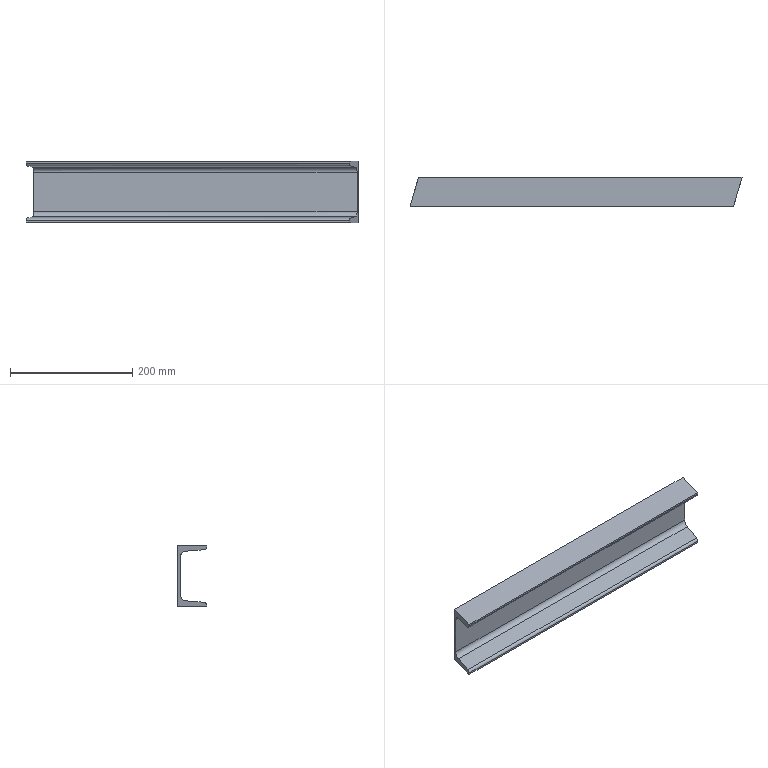Part | STEP file | 12-Channel 100x48_default<machining> | 1 solid | 14 faces | box 544 x 48 x 100 mm | volume 666800 mm3 | plane 10 | cylinder 4 | commonest cylinder face diameters 8.5 x2 17 x2
STEP:
#1=CARTESIAN_POINT('',(0.,0.,0.));
#2=DIRECTION('',(0.,0.,1.));
#3=DIRECTION('',(1.,0.,0.));
#4=AXIS2_PLACEMENT_3D('',#1,#2,#3);
#5=CARTESIAN_POINT('',(544.,0.,-100.));
#6=VERTEX_POINT('',#5);
#7=CARTESIAN_POINT('',(14.,0.,-100.));
#8=VERTEX_POINT('',#7);
#9=CARTESIAN_POINT('',(544.,0.,-100.));
#10=DIRECTION('',(-1.,0.,0.));
#11=VECTOR('',#10,1.);
#12=LINE('',#9,#11);
#13=CARTESIAN_POINT('',(544.,0.,-100.));
#14=DIRECTION('',(0.,0.,1.));
#15=DIRECTION('',(1.,0.,0.));
#16=AXIS2_PLACEMENT_3D('',#13,#14,#15);
#17=PLANE('',#16);
#18=CARTESIAN_POINT('',(0.,0.));
#19=DIRECTION('',(-1.,0.));
#20=VECTOR('',#19,1.);
#21=LINE('',#18,#20);
#22=(GEOMETRIC_REPRESENTATION_CONTEXT(2)PARAMETRIC_REPRESENTATION_CONTEXT()REPRESENTATION_CONTEXT('',''));
#23=DEFINITIONAL_REPRESENTATION('',(#21),#22);
#24=PCURVE('',#17,#23);
#25=CARTESIAN_POINT('',(544.,0.,0.));
#26=DIRECTION('',(0.,-1.,0.));
#27=DIRECTION('',(0.,0.,-1.));
#28=AXIS2_PLACEMENT_3D('',#25,#26,#27);
#29=PLANE('',#28);
#30=CARTESIAN_POINT('',(100.,0.));
#31=DIRECTION('',(0.,-1.));
#32=VECTOR('',#31,1.);
#33=LINE('',#30,#32);
#34=(GEOMETRIC_REPRESENTATION_CONTEXT(2)PARAMETRIC_REPRESENTATION_CONTEXT()REPRESENTATION_CONTEXT('',''));
#35=DEFINITIONAL_REPRESENTATION('',(#33),#34);
#36=PCURVE('',#29,#35);
#37=SURFACE_CURVE('',#12,(#24,#36),.PCURVE_S1.);
#38=EDGE_CURVE('',#6,#8,#37,.T.);
#39=ORIENTED_EDGE('',*,*,#38,.F.);
#40=CARTESIAN_POINT('',(530.,-48.,-100.));
#41=VERTEX_POINT('',#40);
#42=CARTESIAN_POINT('',(544.,0.,-100.));
#43=DIRECTION('',(0.28,0.96,0.));
#44=VECTOR('',#43,1.);
#45=LINE('',#42,#44);
#46=CARTESIAN_POINT('',(0.,0.));
#47=DIRECTION('',(0.28,0.96));
#48=VECTOR('',#47,1.);
#49=LINE('',#46,#48);
#50=(GEOMETRIC_REPRESENTATION_CONTEXT(2)PARAMETRIC_REPRESENTATION_CONTEXT()REPRESENTATION_CONTEXT('',''));
#51=DEFINITIONAL_REPRESENTATION('',(#49),#50);
#52=PCURVE('',#17,#51);
#53=CARTESIAN_POINT('',(544.,0.,0.));
#54=DIRECTION('',(-0.96,0.28,0.));
#55=DIRECTION('',(-0.28,-0.96,0.));
#56=AXIS2_PLACEMENT_3D('',#53,#54,#55);
#57=PLANE('',#56);
#58=CARTESIAN_POINT('',(0.,-100.));
#59=DIRECTION('',(-1.,0.));
#60=VECTOR('',#59,1.);
#61=LINE('',#58,#60);
#62=(GEOMETRIC_REPRESENTATION_CONTEXT(2)PARAMETRIC_REPRESENTATION_CONTEXT()REPRESENTATION_CONTEXT('',''));
#63=DEFINITIONAL_REPRESENTATION('',(#61),#62);
#64=PCURVE('',#57,#63);
#65=SURFACE_CURVE('',#45,(#52,#64),.PCURVE_S1.);
#66=EDGE_CURVE('',#41,#6,#65,.T.);
#67=ORIENTED_EDGE('',*,*,#66,.F.);
#68=CARTESIAN_POINT('',(0.,-48.,-100.));
#69=VERTEX_POINT('',#68);
#70=CARTESIAN_POINT('',(544.,-48.,-100.));
#71=DIRECTION('',(-1.,0.,0.));
#72=VECTOR('',#71,1.);
#73=LINE('',#70,#72);
#74=CARTESIAN_POINT('',(0.,-48.));
#75=DIRECTION('',(-1.,0.));
#76=VECTOR('',#75,1.);
#77=LINE('',#74,#76);
#78=(GEOMETRIC_REPRESENTATION_CONTEXT(2)PARAMETRIC_REPRESENTATION_CONTEXT()REPRESENTATION_CONTEXT('',''));
#79=DEFINITIONAL_REPRESENTATION('',(#77),#78);
#80=PCURVE('',#17,#79);
#81=CARTESIAN_POINT('',(544.,-48.,-97.266));
#82=DIRECTION('',(0.,1.,0.));
#83=DIRECTION('',(0.,0.,1.));
#84=AXIS2_PLACEMENT_3D('',#81,#82,#83);
#85=PLANE('',#84);
#86=CARTESIAN_POINT('',(-2.734,0.));
#87=DIRECTION('',(0.,-1.));
#88=VECTOR('',#87,1.);
#89=LINE('',#86,#88);
#90=(GEOMETRIC_REPRESENTATION_CONTEXT(2)PARAMETRIC_REPRESENTATION_CONTEXT()REPRESENTATION_CONTEXT('',''));
#91=DEFINITIONAL_REPRESENTATION('',(#89),#90);
#92=PCURVE('',#85,#91);
#93=SURFACE_CURVE('',#73,(#80,#92),.PCURVE_S1.);
#94=EDGE_CURVE('',#41,#69,#93,.T.);
#95=ORIENTED_EDGE('',*,*,#94,.T.);
#96=CARTESIAN_POINT('',(0.,-48.,-100.));
#97=DIRECTION('',(-0.28,-0.96,0.));
#98=VECTOR('',#97,1.);
#99=LINE('',#96,#98);
#100=CARTESIAN_POINT('',(-544.,-48.));
#101=DIRECTION('',(-0.28,-0.96));
#102=VECTOR('',#101,1.);
#103=LINE('',#100,#102);
#104=(GEOMETRIC_REPRESENTATION_CONTEXT(2)PARAMETRIC_REPRESENTATION_CONTEXT()REPRESENTATION_CONTEXT('',''));
#105=DEFINITIONAL_REPRESENTATION('',(#103),#104);
#106=PCURVE('',#17,#105);
#107=CARTESIAN_POINT('',(0.,-48.,0.));
#108=DIRECTION('',(0.96,-0.28,0.));
#109=DIRECTION('',(0.28,0.96,0.));
#110=AXIS2_PLACEMENT_3D('',#107,#108,#109);
#111=PLANE('',#110);
#112=CARTESIAN_POINT('',(0.,-100.));
#113=DIRECTION('',(-1.,0.));
#114=VECTOR('',#113,1.);
#115=LINE('',#112,#114);
#116=(GEOMETRIC_REPRESENTATION_CONTEXT(2)PARAMETRIC_REPRESENTATION_CONTEXT()REPRESENTATION_CONTEXT('',''));
#117=DEFINITIONAL_REPRESENTATION('',(#115),#116);
#118=PCURVE('',#111,#117);
#119=SURFACE_CURVE('',#99,(#106,#118),.PCURVE_S1.);
#120=EDGE_CURVE('',#8,#69,#119,.T.);
#121=ORIENTED_EDGE('',*,*,#120,.F.);
#122=EDGE_LOOP('',(#39,#67,#95,#121));
#123=FACE_BOUND('',#122,.T.);
#124=ADVANCED_FACE('',(#123),#17,.F.);
#125=ORIENTED_EDGE('',*,*,#38,.T.);
#126=CARTESIAN_POINT('',(14.,0.,0.));
#127=VERTEX_POINT('',#126);
#128=CARTESIAN_POINT('',(14.,0.,0.));
#129=DIRECTION('',(0.,0.,-1.));
#130=VECTOR('',#129,1.);
#131=LINE('',#128,#130);
#132=CARTESIAN_POINT('',(0.,-530.));
#133=DIRECTION('',(1.,0.));
#134=VECTOR('',#133,1.);
#135=LINE('',#132,#134);
#136=(GEOMETRIC_REPRESENTATION_CONTEXT(2)PARAMETRIC_REPRESENTATION_CONTEXT()REPRESENTATION_CONTEXT('',''));
#137=DEFINITIONAL_REPRESENTATION('',(#135),#136);
#138=PCURVE('',#29,#137);
#139=CARTESIAN_POINT('',(50.,0.));
#140=DIRECTION('',(0.,-1.));
#141=VECTOR('',#140,1.);
#142=LINE('',#139,#141);
#143=(GEOMETRIC_REPRESENTATION_CONTEXT(2)PARAMETRIC_REPRESENTATION_CONTEXT()REPRESENTATION_CONTEXT('',''));
#144=DEFINITIONAL_REPRESENTATION('',(#142),#143);
#145=PCURVE('',#111,#144);
#146=SURFACE_CURVE('',#131,(#138,#145),.PCURVE_S1.);
#147=EDGE_CURVE('',#127,#8,#146,.T.);
#148=ORIENTED_EDGE('',*,*,#147,.F.);
#149=CARTESIAN_POINT('',(544.,0.,0.));
#150=VERTEX_POINT('',#149);
#151=CARTESIAN_POINT('',(544.,0.,0.));
#152=DIRECTION('',(-1.,0.,0.));
#153=VECTOR('',#152,1.);
#154=LINE('',#151,#153);
#155=CARTESIAN_POINT('',(0.,0.));
#156=DIRECTION('',(0.,-1.));
#157=VECTOR('',#156,1.);
#158=LINE('',#155,#157);
#159=(GEOMETRIC_REPRESENTATION_CONTEXT(2)PARAMETRIC_REPRESENTATION_CONTEXT()REPRESENTATION_CONTEXT('',''));
#160=DEFINITIONAL_REPRESENTATION('',(#158),#159);
#161=PCURVE('',#29,#160);
#162=CARTESIAN_POINT('',(544.,0.,0.));
#163=DIRECTION('',(0.,0.,-1.));
#164=DIRECTION('',(0.,1.,0.));
#165=AXIS2_PLACEMENT_3D('',#162,#163,#164);
#166=PLANE('',#165);
#167=CARTESIAN_POINT('',(0.,0.));
#168=DIRECTION('',(0.,-1.));
#169=VECTOR('',#168,1.);
#170=LINE('',#167,#169);
#171=(GEOMETRIC_REPRESENTATION_CONTEXT(2)PARAMETRIC_REPRESENTATION_CONTEXT()REPRESENTATION_CONTEXT('',''));
#172=DEFINITIONAL_REPRESENTATION('',(#170),#171);
#173=PCURVE('',#166,#172);
#174=SURFACE_CURVE('',#154,(#161,#173),.PCURVE_S1.);
#175=EDGE_CURVE('',#150,#127,#174,.T.);
#176=ORIENTED_EDGE('',*,*,#175,.F.);
#177=CARTESIAN_POINT('',(544.,0.,0.));
#178=DIRECTION('',(0.,0.,1.));
#179=VECTOR('',#178,1.);
#180=LINE('',#177,#179);
#181=CARTESIAN_POINT('',(0.,0.));
#182=DIRECTION('',(-1.,0.));
#183=VECTOR('',#182,1.);
#184=LINE('',#181,#183);
#185=(GEOMETRIC_REPRESENTATION_CONTEXT(2)PARAMETRIC_REPRESENTATION_CONTEXT()REPRESENTATION_CONTEXT('',''));
#186=DEFINITIONAL_REPRESENTATION('',(#184),#185);
#187=PCURVE('',#29,#186);
#188=CARTESIAN_POINT('',(0.,0.));
#189=DIRECTION('',(0.,1.));
#190=VECTOR('',#189,1.);
#191=LINE('',#188,#190);
#192=(GEOMETRIC_REPRESENTATION_CONTEXT(2)PARAMETRIC_REPRESENTATION_CONTEXT()REPRESENTATION_CONTEXT('',''));
#193=DEFINITIONAL_REPRESENTATION('',(#191),#192);
#194=PCURVE('',#57,#193);
#195=SURFACE_CURVE('',#180,(#187,#194),.PCURVE_S1.);
#196=EDGE_CURVE('',#6,#150,#195,.T.);
#197=ORIENTED_EDGE('',*,*,#196,.F.);
#198=EDGE_LOOP('',(#125,#148,#176,#197));
#199=FACE_BOUND('',#198,.T.);
#200=ADVANCED_FACE('',(#199),#29,.F.);
#201=CARTESIAN_POINT('',(530.,-48.,0.));
#202=VERTEX_POINT('',#201);
#203=CARTESIAN_POINT('',(0.,-48.,0.));
#204=VERTEX_POINT('',#203);
#205=CARTESIAN_POINT('',(544.,-48.,0.));
#206=DIRECTION('',(-1.,0.,0.));
#207=VECTOR('',#206,1.);
#208=LINE('',#205,#207);
#209=CARTESIAN_POINT('',(-48.,0.));
#210=DIRECTION('',(0.,-1.));
#211=VECTOR('',#210,1.);
#212=LINE('',#209,#211);
#213=(GEOMETRIC_REPRESENTATION_CONTEXT(2)PARAMETRIC_REPRESENTATION_CONTEXT()REPRESENTATION_CONTEXT('',''));
#214=DEFINITIONAL_REPRESENTATION('',(#212),#213);
#215=PCURVE('',#166,#214);
#216=CARTESIAN_POINT('',(544.,-48.,-2.734));
#217=DIRECTION('',(0.,1.,0.));
#218=DIRECTION('',(0.,0.,1.));
#219=AXIS2_PLACEMENT_3D('',#216,#217,#218);
#220=PLANE('',#219);
#221=CARTESIAN_POINT('',(2.734,0.));
#222=DIRECTION('',(0.,-1.));
#223=VECTOR('',#222,1.);
#224=LINE('',#221,#223);
#225=(GEOMETRIC_REPRESENTATION_CONTEXT(2)PARAMETRIC_REPRESENTATION_CONTEXT()REPRESENTATION_CONTEXT('',''));
#226=DEFINITIONAL_REPRESENTATION('',(#224),#225);
#227=PCURVE('',#220,#226);
#228=SURFACE_CURVE('',#208,(#215,#227),.PCURVE_S1.);
#229=EDGE_CURVE('',#202,#204,#228,.T.);
#230=ORIENTED_EDGE('',*,*,#229,.F.);
#231=CARTESIAN_POINT('',(544.,0.,0.));
#232=DIRECTION('',(0.28,0.96,0.));
#233=VECTOR('',#232,1.);
#234=LINE('',#231,#233);
#235=CARTESIAN_POINT('',(0.,0.));
#236=DIRECTION('',(0.96,0.28));
#237=VECTOR('',#236,1.);
#238=LINE('',#235,#237);
#239=(GEOMETRIC_REPRESENTATION_CONTEXT(2)PARAMETRIC_REPRESENTATION_CONTEXT()REPRESENTATION_CONTEXT('',''));
#240=DEFINITIONAL_REPRESENTATION('',(#238),#239);
#241=PCURVE('',#166,#240);
#242=CARTESIAN_POINT('',(0.,0.));
#243=DIRECTION('',(-1.,0.));
#244=VECTOR('',#243,1.);
#245=LINE('',#242,#244);
#246=(GEOMETRIC_REPRESENTATION_CONTEXT(2)PARAMETRIC_REPRESENTATION_CONTEXT()REPRESENTATION_CONTEXT('',''));
#247=DEFINITIONAL_REPRESENTATION('',(#245),#246);
#248=PCURVE('',#57,#247);
#249=SURFACE_CURVE('',#234,(#241,#248),.PCURVE_S1.);
#250=EDGE_CURVE('',#202,#150,#249,.T.);
#251=ORIENTED_EDGE('',*,*,#250,.T.);
#252=ORIENTED_EDGE('',*,*,#175,.T.);
#253=CARTESIAN_POINT('',(0.,-48.,0.));
#254=DIRECTION('',(-0.28,-0.96,0.));
#255=VECTOR('',#254,1.);
#256=LINE('',#253,#255);
#257=CARTESIAN_POINT('',(-48.,-544.));
#258=DIRECTION('',(-0.96,-0.28));
#259=VECTOR('',#258,1.);
#260=LINE('',#257,#259);
#261=(GEOMETRIC_REPRESENTATION_CONTEXT(2)PARAMETRIC_REPRESENTATION_CONTEXT()REPRESENTATION_CONTEXT('',''));
#262=DEFINITIONAL_REPRESENTATION('',(#260),#261);
#263=PCURVE('',#166,#262);
#264=CARTESIAN_POINT('',(0.,0.));
#265=DIRECTION('',(-1.,0.));
#266=VECTOR('',#265,1.);
#267=LINE('',#264,#266);
#268=(GEOMETRIC_REPRESENTATION_CONTEXT(2)PARAMETRIC_REPRESENTATION_CONTEXT()REPRESENTATION_CONTEXT('',''));
#269=DEFINITIONAL_REPRESENTATION('',(#267),#268);
#270=PCURVE('',#111,#269);
#271=SURFACE_CURVE('',#256,(#263,#270),.PCURVE_S1.);
#272=EDGE_CURVE('',#127,#204,#271,.T.);
#273=ORIENTED_EDGE('',*,*,#272,.T.);
#274=EDGE_LOOP('',(#230,#251,#252,#273));
#275=FACE_BOUND('',#274,.T.);
#276=ADVANCED_FACE('',(#275),#166,.F.);
#277=CARTESIAN_POINT('',(530.,-48.,-2.734));
#278=VERTEX_POINT('',#277);
#279=CARTESIAN_POINT('',(0.,-48.,-2.734));
#280=VERTEX_POINT('',#279);
#281=CARTESIAN_POINT('',(544.,-48.,-2.734));
#282=DIRECTION('',(-1.,0.,0.));
#283=VECTOR('',#282,1.);
#284=LINE('',#281,#283);
#285=CARTESIAN_POINT('',(0.,0.));
#286=DIRECTION('',(0.,-1.));
#287=VECTOR('',#286,1.);
#288=LINE('',#285,#287);
#289=(GEOMETRIC_REPRESENTATION_CONTEXT(2)PARAMETRIC_REPRESENTATION_CONTEXT()REPRESENTATION_CONTEXT('',''));
#290=DEFINITIONAL_REPRESENTATION('',(#288),#289);
#291=PCURVE('',#220,#290);
#292=CARTESIAN_POINT('',(544.,-43.75,-2.734));
#293=DIRECTION('',(-1.,0.,0.));
#294=DIRECTION('',(0.,0.,1.));
#295=AXIS2_PLACEMENT_3D('',#292,#293,#294);
#296=CYLINDRICAL_SURFACE('',#295,4.25);
#297=CARTESIAN_POINT('',(4.712,0.));
#298=DIRECTION('',(0.,1.));
#299=VECTOR('',#298,1.);
#300=LINE('',#297,#299);
#301=(GEOMETRIC_REPRESENTATION_CONTEXT(2)PARAMETRIC_REPRESENTATION_CONTEXT()REPRESENTATION_CONTEXT('',''));
#302=DEFINITIONAL_REPRESENTATION('',(#300),#301);
#303=PCURVE('',#296,#302);
#304=SURFACE_CURVE('',#284,(#291,#303),.PCURVE_S1.);
#305=EDGE_CURVE('',#278,#280,#304,.T.);
#306=ORIENTED_EDGE('',*,*,#305,.F.);
#307=CARTESIAN_POINT('',(530.,-48.,0.));
#308=DIRECTION('',(0.,0.,-1.));
#309=VECTOR('',#308,1.);
#310=LINE('',#307,#309);
#311=CARTESIAN_POINT('',(2.734,-14.));
#312=DIRECTION('',(-1.,0.));
#313=VECTOR('',#312,1.);
#314=LINE('',#311,#313);
#315=(GEOMETRIC_REPRESENTATION_CONTEXT(2)PARAMETRIC_REPRESENTATION_CONTEXT()REPRESENTATION_CONTEXT('',''));
#316=DEFINITIONAL_REPRESENTATION('',(#314),#315);
#317=PCURVE('',#220,#316);
#318=CARTESIAN_POINT('',(50.,0.));
#319=DIRECTION('',(0.,-1.));
#320=VECTOR('',#319,1.);
#321=LINE('',#318,#320);
#322=(GEOMETRIC_REPRESENTATION_CONTEXT(2)PARAMETRIC_REPRESENTATION_CONTEXT()REPRESENTATION_CONTEXT('',''));
#323=DEFINITIONAL_REPRESENTATION('',(#321),#322);
#324=PCURVE('',#57,#323);
#325=SURFACE_CURVE('',#310,(#317,#324),.PCURVE_S1.);
#326=EDGE_CURVE('',#202,#278,#325,.T.);
#327=ORIENTED_EDGE('',*,*,#326,.F.);
#328=ORIENTED_EDGE('',*,*,#229,.T.);
#329=CARTESIAN_POINT('',(0.,-48.,-2.734));
#330=DIRECTION('',(0.,0.,-1.));
#331=VECTOR('',#330,1.);
#332=LINE('',#329,#331);
#333=CARTESIAN_POINT('',(0.,-544.));
#334=DIRECTION('',(-1.,0.));
#335=VECTOR('',#334,1.);
#336=LINE('',#333,#335);
#337=(GEOMETRIC_REPRESENTATION_CONTEXT(2)PARAMETRIC_REPRESENTATION_CONTEXT()REPRESENTATION_CONTEXT('',''));
#338=DEFINITIONAL_REPRESENTATION('',(#336),#337);
#339=PCURVE('',#220,#338);
#340=CARTESIAN_POINT('',(0.,-2.734));
#341=DIRECTION('',(0.,-1.));
#342=VECTOR('',#341,1.);
#343=LINE('',#340,#342);
#344=(GEOMETRIC_REPRESENTATION_CONTEXT(2)PARAMETRIC_REPRESENTATION_CONTEXT()REPRESENTATION_CONTEXT('',''));
#345=DEFINITIONAL_REPRESENTATION('',(#343),#344);
#346=PCURVE('',#111,#345);
#347=SURFACE_CURVE('',#332,(#339,#346),.PCURVE_S1.);
#348=EDGE_CURVE('',#204,#280,#347,.T.);
#349=ORIENTED_EDGE('',*,*,#348,.T.);
#350=EDGE_LOOP('',(#306,#327,#328,#349));
#351=FACE_BOUND('',#350,.T.);
#352=ADVANCED_FACE('',(#351),#220,.F.);
#353=CARTESIAN_POINT('',(531.146,-44.073,-6.972));
#354=VERTEX_POINT('',#353);
#355=CARTESIAN_POINT('',(1.146,-44.073,-6.972));
#356=VERTEX_POINT('',#355);
#357=CARTESIAN_POINT('',(544.,-44.073,-6.972));
#358=DIRECTION('',(-1.,0.,0.));
#359=VECTOR('',#358,1.);
#360=LINE('',#357,#359);
#361=CARTESIAN_POINT('',(3.218,0.));
#362=DIRECTION('',(0.,1.));
#363=VECTOR('',#362,1.);
#364=LINE('',#361,#363);
#365=(GEOMETRIC_REPRESENTATION_CONTEXT(2)PARAMETRIC_REPRESENTATION_CONTEXT()REPRESENTATION_CONTEXT('',''));
#366=DEFINITIONAL_REPRESENTATION('',(#364),#365);
#367=PCURVE('',#296,#366);
#368=CARTESIAN_POINT('',(544.,-13.155,-9.325));
#369=DIRECTION('',(0.,0.07589,0.9971));
#370=DIRECTION('',(0.,-0.9971,0.07589));
#371=AXIS2_PLACEMENT_3D('',#368,#369,#370);
#372=PLANE('',#371);
#373=CARTESIAN_POINT('',(31.007,0.));
#374=DIRECTION('',(0.,-1.));
#375=VECTOR('',#374,1.);
#376=LINE('',#373,#375);
#377=(GEOMETRIC_REPRESENTATION_CONTEXT(2)PARAMETRIC_REPRESENTATION_CONTEXT()REPRESENTATION_CONTEXT('',''));
#378=DEFINITIONAL_REPRESENTATION('',(#376),#377);
#379=PCURVE('',#372,#378);
#380=SURFACE_CURVE('',#360,(#367,#379),.PCURVE_S1.);
#381=EDGE_CURVE('',#354,#356,#380,.T.);
#382=ORIENTED_EDGE('',*,*,#381,.F.);
#383=CARTESIAN_POINT('',(531.146,-44.073,-6.972));
#384=CARTESIAN_POINT('',(530.464,-46.408,-6.794));
#385=CARTESIAN_POINT('',(530.,-48.,-5.077));
#386=CARTESIAN_POINT('',(530.,-48.,-2.734));
#387=(BOUNDED_CURVE()B_SPLINE_CURVE(3,(#383,#384,#385,#386),.UNSPECIFIED.,.F.,.F.)B_SPLINE_CURVE_WITH_KNOTS((4,4),(4.788,6.283),.PIECEWISE_BEZIER_KNOTS.)CURVE()GEOMETRIC_REPRESENTATION_ITEM()RATIONAL_B_SPLINE_CURVE((1.,0.8223,0.8223,1.))REPRESENTATION_ITEM(''));
#388=CARTESIAN_POINT('',(3.218,12.854));
#389=CARTESIAN_POINT('',(3.238,12.88));
#390=CARTESIAN_POINT('',(3.28,12.931));
#391=CARTESIAN_POINT('',(3.344,13.01));
#392=CARTESIAN_POINT('',(3.409,13.088));
#393=CARTESIAN_POINT('',(3.476,13.167));
#394=CARTESIAN_POINT('',(3.543,13.246));
#395=CARTESIAN_POINT('',(3.612,13.323));
#396=CARTESIAN_POINT('',(3.682,13.398));
#397=CARTESIAN_POINT('',(3.752,13.471));
#398=CARTESIAN_POINT('',(3.823,13.541));
#399=CARTESIAN_POINT('',(3.894,13.608));
#400=CARTESIAN_POINT('',(3.965,13.67));
#401=CARTESIAN_POINT('',(4.036,13.728));
#402=CARTESIAN_POINT('',(4.107,13.781));
#403=CARTESIAN_POINT('',(4.178,13.828));
#404=CARTESIAN_POINT('',(4.248,13.87));
#405=CARTESIAN_POINT('',(4.318,13.906));
#406=CARTESIAN_POINT('',(4.387,13.936));
#407=CARTESIAN_POINT('',(4.454,13.96));
#408=CARTESIAN_POINT('',(4.521,13.978));
#409=CARTESIAN_POINT('',(4.586,13.991));
#410=CARTESIAN_POINT('',(4.65,13.998));
#411=CARTESIAN_POINT('',(4.692,14.));
#412=CARTESIAN_POINT('',(4.712,14.));
#413=B_SPLINE_CURVE_WITH_KNOTS('',3,(#388,#389,#390,#391,#392,#393,#394,#395,#396,#397,#398,#399,#400,#401,#402,#403,#404,#405,#406,#407,#408,#409,#410,#411,#412),.UNSPECIFIED.,.F.,.F.,(4,1,1,1,1,1,1,1,1,1,1,1,1,1,1,1,1,1,1,1,1,1,4),(4.788,4.856,4.924,4.992,5.06,5.128,5.196,5.264,5.332,5.4,5.468,5.536,5.604,5.672,5.74,5.808,5.876,5.943,6.011,6.079,6.147,6.215,6.283),.QUASI_UNIFORM_KNOTS.);
#414=(GEOMETRIC_REPRESENTATION_CONTEXT(2)PARAMETRIC_REPRESENTATION_CONTEXT()REPRESENTATION_CONTEXT('',''));
#415=DEFINITIONAL_REPRESENTATION('',(#413),#414);
#416=PCURVE('',#296,#415);
#417=CARTESIAN_POINT('',(45.909,-6.972));
#418=CARTESIAN_POINT('',(48.342,-6.794));
#419=CARTESIAN_POINT('',(50.,-5.077));
#420=CARTESIAN_POINT('',(50.,-2.734));
#421=(BOUNDED_CURVE()B_SPLINE_CURVE(3,(#417,#418,#419,#420),.UNSPECIFIED.,.F.,.F.)B_SPLINE_CURVE_WITH_KNOTS((4,4),(4.788,6.283),.PIECEWISE_BEZIER_KNOTS.)CURVE()GEOMETRIC_REPRESENTATION_ITEM()RATIONAL_B_SPLINE_CURVE((1.,0.8223,0.8223,1.))REPRESENTATION_ITEM(''));
#422=(GEOMETRIC_REPRESENTATION_CONTEXT(2)PARAMETRIC_REPRESENTATION_CONTEXT()REPRESENTATION_CONTEXT('',''));
#423=DEFINITIONAL_REPRESENTATION('',(#421),#422);
#424=PCURVE('',#57,#423);
#425=SURFACE_CURVE('',#387,(#416,#424),.PCURVE_S1.);
#426=EDGE_CURVE('',#354,#278,#425,.T.);
#427=ORIENTED_EDGE('',*,*,#426,.T.);
#428=ORIENTED_EDGE('',*,*,#305,.T.);
#429=CARTESIAN_POINT('',(0.,-48.,-2.734));
#430=CARTESIAN_POINT('',(0.,-48.,-5.077));
#431=CARTESIAN_POINT('',(0.4644,-46.408,-6.794));
#432=CARTESIAN_POINT('',(1.146,-44.073,-6.972));
#433=(BOUNDED_CURVE()B_SPLINE_CURVE(3,(#429,#430,#431,#432),.UNSPECIFIED.,.F.,.F.)B_SPLINE_CURVE_WITH_KNOTS((4,4),(0.,1.495),.PIECEWISE_BEZIER_KNOTS.)CURVE()GEOMETRIC_REPRESENTATION_ITEM()RATIONAL_B_SPLINE_CURVE((1.,0.8223,0.8223,1.))REPRESENTATION_ITEM(''));
#434=CARTESIAN_POINT('',(4.712,544.));
#435=CARTESIAN_POINT('',(4.692,544.));
#436=CARTESIAN_POINT('',(4.65,543.998));
#437=CARTESIAN_POINT('',(4.586,543.991));
#438=CARTESIAN_POINT('',(4.521,543.978));
#439=CARTESIAN_POINT('',(4.454,543.96));
#440=CARTESIAN_POINT('',(4.387,543.936));
#441=CARTESIAN_POINT('',(4.318,543.906));
#442=CARTESIAN_POINT('',(4.248,543.87));
#443=CARTESIAN_POINT('',(4.178,543.828));
#444=CARTESIAN_POINT('',(4.107,543.781));
#445=CARTESIAN_POINT('',(4.036,543.728));
#446=CARTESIAN_POINT('',(3.965,543.67));
#447=CARTESIAN_POINT('',(3.894,543.608));
#448=CARTESIAN_POINT('',(3.823,543.541));
#449=CARTESIAN_POINT('',(3.752,543.471));
#450=CARTESIAN_POINT('',(3.682,543.398));
#451=CARTESIAN_POINT('',(3.612,543.323));
#452=CARTESIAN_POINT('',(3.543,543.246));
#453=CARTESIAN_POINT('',(3.476,543.167));
#454=CARTESIAN_POINT('',(3.409,543.088));
#455=CARTESIAN_POINT('',(3.344,543.01));
#456=CARTESIAN_POINT('',(3.28,542.931));
#457=CARTESIAN_POINT('',(3.238,542.88));
#458=CARTESIAN_POINT('',(3.218,542.854));
#459=B_SPLINE_CURVE_WITH_KNOTS('',3,(#434,#435,#436,#437,#438,#439,#440,#441,#442,#443,#444,#445,#446,#447,#448,#449,#450,#451,#452,#453,#454,#455,#456,#457,#458),.UNSPECIFIED.,.F.,.F.,(4,1,1,1,1,1,1,1,1,1,1,1,1,1,1,1,1,1,1,1,1,1,4),(0.,0.06795,0.1359,0.2038,0.2718,0.3397,0.4077,0.4756,0.5436,0.6115,0.6795,0.7474,0.8154,0.8833,0.9513,1.019,1.087,1.155,1.223,1.291,1.359,1.427,1.495),.QUASI_UNIFORM_KNOTS.);
#460=(GEOMETRIC_REPRESENTATION_CONTEXT(2)PARAMETRIC_REPRESENTATION_CONTEXT()REPRESENTATION_CONTEXT('',''));
#461=DEFINITIONAL_REPRESENTATION('',(#459),#460);
#462=PCURVE('',#296,#461);
#463=CARTESIAN_POINT('',(0.,-2.734));
#464=CARTESIAN_POINT('',(0.,-5.077));
#465=CARTESIAN_POINT('',(1.658,-6.794));
#466=CARTESIAN_POINT('',(4.091,-6.972));
#467=(BOUNDED_CURVE()B_SPLINE_CURVE(3,(#463,#464,#465,#466),.UNSPECIFIED.,.F.,.F.)B_SPLINE_CURVE_WITH_KNOTS((4,4),(0.,1.495),.PIECEWISE_BEZIER_KNOTS.)CURVE()GEOMETRIC_REPRESENTATION_ITEM()RATIONAL_B_SPLINE_CURVE((1.,0.8223,0.8223,1.))REPRESENTATION_ITEM(''));
#468=(GEOMETRIC_REPRESENTATION_CONTEXT(2)PARAMETRIC_REPRESENTATION_CONTEXT()REPRESENTATION_CONTEXT('',''));
#469=DEFINITIONAL_REPRESENTATION('',(#467),#468);
#470=PCURVE('',#111,#469);
#471=SURFACE_CURVE('',#433,(#462,#470),.PCURVE_S1.);
#472=EDGE_CURVE('',#280,#356,#471,.T.);
#473=ORIENTED_EDGE('',*,*,#472,.T.);
#474=EDGE_LOOP('',(#382,#427,#428,#473));
#475=FACE_BOUND('',#474,.T.);
#476=ADVANCED_FACE('',(#475),#296,.T.);
#477=CARTESIAN_POINT('',(540.163,-13.155,-9.325));
#478=VERTEX_POINT('',#477);
#479=CARTESIAN_POINT('',(10.163,-13.155,-9.325));
#480=VERTEX_POINT('',#479);
#481=CARTESIAN_POINT('',(544.,-13.155,-9.325));
#482=DIRECTION('',(-1.,0.,0.));
#483=VECTOR('',#482,1.);
#484=LINE('',#481,#483);
#485=CARTESIAN_POINT('',(0.,0.));
#486=DIRECTION('',(0.,-1.));
#487=VECTOR('',#486,1.);
#488=LINE('',#485,#487);
#489=(GEOMETRIC_REPRESENTATION_CONTEXT(2)PARAMETRIC_REPRESENTATION_CONTEXT()REPRESENTATION_CONTEXT('',''));
#490=DEFINITIONAL_REPRESENTATION('',(#488),#489);
#491=PCURVE('',#372,#490);
#492=CARTESIAN_POINT('',(544.,-13.8,-17.801));
#493=DIRECTION('',(-1.,0.,0.));
#494=DIRECTION('',(0.,0.,1.));
#495=AXIS2_PLACEMENT_3D('',#492,#493,#494);
#496=CYLINDRICAL_SURFACE('',#495,8.5);
#497=CARTESIAN_POINT('',(0.07597,0.));
#498=DIRECTION('',(0.,1.));
#499=VECTOR('',#498,1.);
#500=LINE('',#497,#499);
#501=(GEOMETRIC_REPRESENTATION_CONTEXT(2)PARAMETRIC_REPRESENTATION_CONTEXT()REPRESENTATION_CONTEXT('',''));
#502=DEFINITIONAL_REPRESENTATION('',(#500),#501);
#503=PCURVE('',#496,#502);
#504=SURFACE_CURVE('',#484,(#491,#503),.PCURVE_S1.);
#505=EDGE_CURVE('',#478,#480,#504,.T.);
#506=ORIENTED_EDGE('',*,*,#505,.F.);
#507=CARTESIAN_POINT('',(540.462,-12.129,-9.404));
#508=DIRECTION('',(-0.2793,-0.9574,0.07287));
#509=VECTOR('',#508,1.);
#510=LINE('',#507,#509);
#511=CARTESIAN_POINT('',(-1.029,-3.538));
#512=DIRECTION('',(0.9602,-0.2793));
#513=VECTOR('',#512,1.);
#514=LINE('',#511,#513);
#515=(GEOMETRIC_REPRESENTATION_CONTEXT(2)PARAMETRIC_REPRESENTATION_CONTEXT()REPRESENTATION_CONTEXT('',''));
#516=DEFINITIONAL_REPRESENTATION('',(#514),#515);
#517=PCURVE('',#372,#516);
#518=CARTESIAN_POINT('',(12.634,-9.404));
#519=DIRECTION('',(0.9973,0.07287));
#520=VECTOR('',#519,1.);
#521=LINE('',#518,#520);
#522=(GEOMETRIC_REPRESENTATION_CONTEXT(2)PARAMETRIC_REPRESENTATION_CONTEXT()REPRESENTATION_CONTEXT('',''));
#523=DEFINITIONAL_REPRESENTATION('',(#521),#522);
#524=PCURVE('',#57,#523);
#525=SURFACE_CURVE('',#510,(#517,#524),.PCURVE_S1.);
#526=EDGE_CURVE('',#478,#354,#525,.T.);
#527=ORIENTED_EDGE('',*,*,#526,.T.);
#528=ORIENTED_EDGE('',*,*,#381,.T.);
#529=CARTESIAN_POINT('',(51.794,129.578,-20.189));
#530=DIRECTION('',(0.2793,0.9574,-0.07287));
#531=VECTOR('',#530,1.);
#532=LINE('',#529,#531);
#533=CARTESIAN_POINT('',(-143.146,-492.206));
#534=DIRECTION('',(-0.9602,0.2793));
#535=VECTOR('',#534,1.);
#536=LINE('',#533,#535);
#537=(GEOMETRIC_REPRESENTATION_CONTEXT(2)PARAMETRIC_REPRESENTATION_CONTEXT()REPRESENTATION_CONTEXT('',''));
#538=DEFINITIONAL_REPRESENTATION('',(#536),#537);
#539=PCURVE('',#372,#538);
#540=CARTESIAN_POINT('',(184.977,-20.189));
#541=DIRECTION('',(0.9973,-0.07287));
#542=VECTOR('',#541,1.);
#543=LINE('',#540,#542);
#544=(GEOMETRIC_REPRESENTATION_CONTEXT(2)PARAMETRIC_REPRESENTATION_CONTEXT()REPRESENTATION_CONTEXT('',''));
#545=DEFINITIONAL_REPRESENTATION('',(#543),#544);
#546=PCURVE('',#111,#545);
#547=SURFACE_CURVE('',#532,(#539,#546),.PCURVE_S1.);
#548=EDGE_CURVE('',#356,#480,#547,.T.);
#549=ORIENTED_EDGE('',*,*,#548,.T.);
#550=EDGE_LOOP('',(#506,#527,#528,#549));
#551=FACE_BOUND('',#550,.T.);
#552=ADVANCED_FACE('',(#551),#372,.F.);
#553=CARTESIAN_POINT('',(12.454,-5.3,-17.801));
#554=VERTEX_POINT('',#553);
#555=CARTESIAN_POINT('',(10.163,-13.155,-9.325));
#556=CARTESIAN_POINT('',(11.525,-8.484,-9.681));
#557=CARTESIAN_POINT('',(12.454,-5.3,-13.117));
#558=CARTESIAN_POINT('',(12.454,-5.3,-17.801));
#559=(BOUNDED_CURVE()B_SPLINE_CURVE(3,(#555,#556,#557,#558),.UNSPECIFIED.,.F.,.F.)B_SPLINE_CURVE_WITH_KNOTS((4,4),(1.647,3.142),.PIECEWISE_BEZIER_KNOTS.)CURVE()GEOMETRIC_REPRESENTATION_ITEM()RATIONAL_B_SPLINE_CURVE((1.,0.8223,0.8223,1.))REPRESENTATION_ITEM(''));
#560=CARTESIAN_POINT('',(0.07597,533.837));
#561=CARTESIAN_POINT('',(0.09656,533.786));
#562=CARTESIAN_POINT('',(0.1383,533.683));
#563=CARTESIAN_POINT('',(0.2022,533.527));
#564=CARTESIAN_POINT('',(0.2675,533.369));
#565=CARTESIAN_POINT('',(0.3341,533.211));
#566=CARTESIAN_POINT('',(0.4018,533.055));
#567=CARTESIAN_POINT('',(0.4705,532.9));
#568=CARTESIAN_POINT('',(0.54,532.749));
#569=CARTESIAN_POINT('',(0.6102,532.603));
#570=CARTESIAN_POINT('',(0.681,532.463));
#571=CARTESIAN_POINT('',(0.7521,532.33));
#572=CARTESIAN_POINT('',(0.8234,532.205));
#573=CARTESIAN_POINT('',(0.8947,532.09));
#574=CARTESIAN_POINT('',(0.9658,531.984));
#575=CARTESIAN_POINT('',(1.037,531.89));
#576=CARTESIAN_POINT('',(1.107,531.806));
#577=CARTESIAN_POINT('',(1.176,531.734));
#578=CARTESIAN_POINT('',(1.245,531.674));
#579=CARTESIAN_POINT('',(1.313,531.626));
#580=CARTESIAN_POINT('',(1.379,531.589));
#581=CARTESIAN_POINT('',(1.445,531.564));
#582=CARTESIAN_POINT('',(1.509,531.549));
#583=CARTESIAN_POINT('',(1.55,531.546));
#584=CARTESIAN_POINT('',(1.571,531.546));
#585=B_SPLINE_CURVE_WITH_KNOTS('',3,(#560,#561,#562,#563,#564,#565,#566,#567,#568,#569,#570,#571,#572,#573,#574,#575,#576,#577,#578,#579,#580,#581,#582,#583,#584),.UNSPECIFIED.,.F.,.F.,(4,1,1,1,1,1,1,1,1,1,1,1,1,1,1,1,1,1,1,1,1,1,4),(1.647,1.715,1.783,1.851,1.919,1.986,2.054,2.122,2.19,2.258,2.326,2.394,2.462,2.53,2.598,2.666,2.734,2.802,2.87,2.938,3.006,3.074,3.142),.QUASI_UNIFORM_KNOTS.);
#586=(GEOMETRIC_REPRESENTATION_CONTEXT(2)PARAMETRIC_REPRESENTATION_CONTEXT()REPRESENTATION_CONTEXT('',''));
#587=DEFINITIONAL_REPRESENTATION('',(#585),#586);
#588=PCURVE('',#496,#587);
#589=CARTESIAN_POINT('',(36.297,-9.325));
#590=CARTESIAN_POINT('',(41.162,-9.681));
#591=CARTESIAN_POINT('',(44.479,-13.117));
#592=CARTESIAN_POINT('',(44.479,-17.801));
#593=(BOUNDED_CURVE()B_SPLINE_CURVE(3,(#589,#590,#591,#592),.UNSPECIFIED.,.F.,.F.)B_SPLINE_CURVE_WITH_KNOTS((4,4),(1.647,3.142),.PIECEWISE_BEZIER_KNOTS.)CURVE()GEOMETRIC_REPRESENTATION_ITEM()RATIONAL_B_SPLINE_CURVE((1.,0.8223,0.8223,1.))REPRESENTATION_ITEM(''));
#594=(GEOMETRIC_REPRESENTATION_CONTEXT(2)PARAMETRIC_REPRESENTATION_CONTEXT()REPRESENTATION_CONTEXT('',''));
#595=DEFINITIONAL_REPRESENTATION('',(#593),#594);
#596=PCURVE('',#111,#595);
#597=SURFACE_CURVE('',#559,(#588,#596),.PCURVE_S1.);
#598=EDGE_CURVE('',#480,#554,#597,.T.);
#599=ORIENTED_EDGE('',*,*,#598,.F.);
#600=ORIENTED_EDGE('',*,*,#505,.F.);
#601=CARTESIAN_POINT('',(542.454,-5.3,-17.801));
#602=VERTEX_POINT('',#601);
#603=CARTESIAN_POINT('',(542.454,-5.3,-17.801));
#604=CARTESIAN_POINT('',(542.454,-5.3,-13.117));
#605=CARTESIAN_POINT('',(541.525,-8.484,-9.681));
#606=CARTESIAN_POINT('',(540.163,-13.155,-9.325));
#607=(BOUNDED_CURVE()B_SPLINE_CURVE(3,(#603,#604,#605,#606),.UNSPECIFIED.,.F.,.F.)B_SPLINE_CURVE_WITH_KNOTS((4,4),(3.142,4.636),.PIECEWISE_BEZIER_KNOTS.)CURVE()GEOMETRIC_REPRESENTATION_ITEM()RATIONAL_B_SPLINE_CURVE((1.,0.8223,0.8223,1.))REPRESENTATION_ITEM(''));
#608=CARTESIAN_POINT('',(1.571,1.546));
#609=CARTESIAN_POINT('',(1.55,1.546));
#610=CARTESIAN_POINT('',(1.509,1.549));
#611=CARTESIAN_POINT('',(1.445,1.564));
#612=CARTESIAN_POINT('',(1.379,1.589));
#613=CARTESIAN_POINT('',(1.313,1.626));
#614=CARTESIAN_POINT('',(1.245,1.674));
#615=CARTESIAN_POINT('',(1.176,1.734));
#616=CARTESIAN_POINT('',(1.107,1.806));
#617=CARTESIAN_POINT('',(1.037,1.89));
#618=CARTESIAN_POINT('',(0.9658,1.984));
#619=CARTESIAN_POINT('',(0.8947,2.09));
#620=CARTESIAN_POINT('',(0.8234,2.205));
#621=CARTESIAN_POINT('',(0.7521,2.33));
#622=CARTESIAN_POINT('',(0.681,2.463));
#623=CARTESIAN_POINT('',(0.6102,2.603));
#624=CARTESIAN_POINT('',(0.54,2.749));
#625=CARTESIAN_POINT('',(0.4705,2.9));
#626=CARTESIAN_POINT('',(0.4018,3.055));
#627=CARTESIAN_POINT('',(0.3341,3.211));
#628=CARTESIAN_POINT('',(0.2675,3.369));
#629=CARTESIAN_POINT('',(0.2022,3.527));
#630=CARTESIAN_POINT('',(0.1383,3.683));
#631=CARTESIAN_POINT('',(0.09656,3.786));
#632=CARTESIAN_POINT('',(0.07597,3.837));
#633=B_SPLINE_CURVE_WITH_KNOTS('',3,(#608,#609,#610,#611,#612,#613,#614,#615,#616,#617,#618,#619,#620,#621,#622,#623,#624,#625,#626,#627,#628,#629,#630,#631,#632),.UNSPECIFIED.,.F.,.F.,(4,1,1,1,1,1,1,1,1,1,1,1,1,1,1,1,1,1,1,1,1,1,4),(3.142,3.21,3.277,3.345,3.413,3.481,3.549,3.617,3.685,3.753,3.821,3.889,3.957,4.025,4.093,4.161,4.229,4.297,4.365,4.433,4.501,4.568,4.636),.QUASI_UNIFORM_KNOTS.);
#634=(GEOMETRIC_REPRESENTATION_CONTEXT(2)PARAMETRIC_REPRESENTATION_CONTEXT()REPRESENTATION_CONTEXT('',''));
#635=DEFINITIONAL_REPRESENTATION('',(#633),#634);
#636=PCURVE('',#496,#635);
#637=CARTESIAN_POINT('',(5.521,-17.801));
#638=CARTESIAN_POINT('',(5.521,-13.117));
#639=CARTESIAN_POINT('',(8.838,-9.681));
#640=CARTESIAN_POINT('',(13.703,-9.325));
#641=(BOUNDED_CURVE()B_SPLINE_CURVE(3,(#637,#638,#639,#640),.UNSPECIFIED.,.F.,.F.)B_SPLINE_CURVE_WITH_KNOTS((4,4),(3.142,4.636),.PIECEWISE_BEZIER_KNOTS.)CURVE()GEOMETRIC_REPRESENTATION_ITEM()RATIONAL_B_SPLINE_CURVE((1.,0.8223,0.8223,1.))REPRESENTATION_ITEM(''));
#642=(GEOMETRIC_REPRESENTATION_CONTEXT(2)PARAMETRIC_REPRESENTATION_CONTEXT()REPRESENTATION_CONTEXT('',''));
#643=DEFINITIONAL_REPRESENTATION('',(#641),#642);
#644=PCURVE('',#57,#643);
#645=SURFACE_CURVE('',#607,(#636,#644),.PCURVE_S1.);
#646=EDGE_CURVE('',#602,#478,#645,.T.);
#647=ORIENTED_EDGE('',*,*,#646,.F.);
#648=CARTESIAN_POINT('',(544.,-5.3,-17.801));
#649=DIRECTION('',(-1.,0.,0.));
#650=VECTOR('',#649,1.);
#651=LINE('',#648,#650);
#652=CARTESIAN_POINT('',(1.571,0.));
#653=DIRECTION('',(0.,1.));
#654=VECTOR('',#653,1.);
#655=LINE('',#652,#654);
#656=(GEOMETRIC_REPRESENTATION_CONTEXT(2)PARAMETRIC_REPRESENTATION_CONTEXT()REPRESENTATION_CONTEXT('',''));
#657=DEFINITIONAL_REPRESENTATION('',(#655),#656);
#658=PCURVE('',#496,#657);
#659=CARTESIAN_POINT('',(544.,-5.3,-82.199));
#660=DIRECTION('',(0.,1.,0.));
#661=DIRECTION('',(0.,0.,1.));
#662=AXIS2_PLACEMENT_3D('',#659,#660,#661);
#663=PLANE('',#662);
#664=CARTESIAN_POINT('',(64.398,0.));
#665=DIRECTION('',(0.,-1.));
#666=VECTOR('',#665,1.);
#667=LINE('',#664,#666);
#668=(GEOMETRIC_REPRESENTATION_CONTEXT(2)PARAMETRIC_REPRESENTATION_CONTEXT()REPRESENTATION_CONTEXT('',''));
#669=DEFINITIONAL_REPRESENTATION('',(#667),#668);
#670=PCURVE('',#663,#669);
#671=SURFACE_CURVE('',#651,(#658,#670),.PCURVE_S1.);
#672=EDGE_CURVE('',#602,#554,#671,.T.);
#673=ORIENTED_EDGE('',*,*,#672,.T.);
#674=EDGE_LOOP('',(#599,#600,#647,#673));
#675=FACE_BOUND('',#674,.F.);
#676=ADVANCED_FACE('',(#675),#496,.F.);
#677=CARTESIAN_POINT('',(542.454,-5.3,-82.199));
#678=VERTEX_POINT('',#677);
#679=CARTESIAN_POINT('',(12.454,-5.3,-82.199));
#680=VERTEX_POINT('',#679);
#681=CARTESIAN_POINT('',(544.,-5.3,-82.199));
#682=DIRECTION('',(-1.,0.,0.));
#683=VECTOR('',#682,1.);
#684=LINE('',#681,#683);
#685=CARTESIAN_POINT('',(0.,0.));
#686=DIRECTION('',(0.,-1.));
#687=VECTOR('',#686,1.);
#688=LINE('',#685,#687);
#689=(GEOMETRIC_REPRESENTATION_CONTEXT(2)PARAMETRIC_REPRESENTATION_CONTEXT()REPRESENTATION_CONTEXT('',''));
#690=DEFINITIONAL_REPRESENTATION('',(#688),#689);
#691=PCURVE('',#663,#690);
#692=CARTESIAN_POINT('',(544.,-13.8,-82.199));
#693=DIRECTION('',(-1.,0.,0.));
#694=DIRECTION('',(0.,0.,1.));
#695=AXIS2_PLACEMENT_3D('',#692,#693,#694);
#696=CYLINDRICAL_SURFACE('',#695,8.5);
#697=CARTESIAN_POINT('',(1.571,0.));
#698=DIRECTION('',(0.,1.));
#699=VECTOR('',#698,1.);
#700=LINE('',#697,#699);
#701=(GEOMETRIC_REPRESENTATION_CONTEXT(2)PARAMETRIC_REPRESENTATION_CONTEXT()REPRESENTATION_CONTEXT('',''));
#702=DEFINITIONAL_REPRESENTATION('',(#700),#701);
#703=PCURVE('',#696,#702);
#704=SURFACE_CURVE('',#684,(#691,#703),.PCURVE_S1.);
#705=EDGE_CURVE('',#678,#680,#704,.T.);
#706=ORIENTED_EDGE('',*,*,#705,.F.);
#707=CARTESIAN_POINT('',(542.454,-5.3,-82.199));
#708=DIRECTION('',(0.,0.,1.));
#709=VECTOR('',#708,1.);
#710=LINE('',#707,#709);
#711=CARTESIAN_POINT('',(0.,-1.546));
#712=DIRECTION('',(1.,0.));
#713=VECTOR('',#712,1.);
#714=LINE('',#711,#713);
#715=(GEOMETRIC_REPRESENTATION_CONTEXT(2)PARAMETRIC_REPRESENTATION_CONTEXT()REPRESENTATION_CONTEXT('',''));
#716=DEFINITIONAL_REPRESENTATION('',(#714),#715);
#717=PCURVE('',#663,#716);
#718=CARTESIAN_POINT('',(5.521,-82.199));
#719=DIRECTION('',(0.,1.));
#720=VECTOR('',#719,1.);
#721=LINE('',#718,#720);
#722=(GEOMETRIC_REPRESENTATION_CONTEXT(2)PARAMETRIC_REPRESENTATION_CONTEXT()REPRESENTATION_CONTEXT('',''));
#723=DEFINITIONAL_REPRESENTATION('',(#721),#722);
#724=PCURVE('',#57,#723);
#725=SURFACE_CURVE('',#710,(#717,#724),.PCURVE_S1.);
#726=EDGE_CURVE('',#678,#602,#725,.T.);
#727=ORIENTED_EDGE('',*,*,#726,.T.);
#728=ORIENTED_EDGE('',*,*,#672,.T.);
#729=CARTESIAN_POINT('',(12.454,-5.3,-82.199));
#730=DIRECTION('',(0.,0.,-1.));
#731=VECTOR('',#730,1.);
#732=LINE('',#729,#731);
#733=CARTESIAN_POINT('',(0.,-531.546));
#734=DIRECTION('',(-1.,0.));
#735=VECTOR('',#734,1.);
#736=LINE('',#733,#735);
#737=(GEOMETRIC_REPRESENTATION_CONTEXT(2)PARAMETRIC_REPRESENTATION_CONTEXT()REPRESENTATION_CONTEXT('',''));
#738=DEFINITIONAL_REPRESENTATION('',(#736),#737);
#739=PCURVE('',#663,#738);
#740=CARTESIAN_POINT('',(44.479,-82.199));
#741=DIRECTION('',(0.,-1.));
#742=VECTOR('',#741,1.);
#743=LINE('',#740,#742);
#744=(GEOMETRIC_REPRESENTATION_CONTEXT(2)PARAMETRIC_REPRESENTATION_CONTEXT()REPRESENTATION_CONTEXT('',''));
#745=DEFINITIONAL_REPRESENTATION('',(#743),#744);
#746=PCURVE('',#111,#745);
#747=SURFACE_CURVE('',#732,(#739,#746),.PCURVE_S1.);
#748=EDGE_CURVE('',#554,#680,#747,.T.);
#749=ORIENTED_EDGE('',*,*,#748,.T.);
#750=EDGE_LOOP('',(#706,#727,#728,#749));
#751=FACE_BOUND('',#750,.T.);
#752=ADVANCED_FACE('',(#751),#663,.F.);
#753=CARTESIAN_POINT('',(10.163,-13.155,-90.675));
#754=VERTEX_POINT('',#753);
#755=CARTESIAN_POINT('',(12.454,-5.3,-82.199));
#756=CARTESIAN_POINT('',(12.454,-5.3,-86.883));
#757=CARTESIAN_POINT('',(11.525,-8.484,-90.319));
#758=CARTESIAN_POINT('',(10.163,-13.155,-90.675));
#759=(BOUNDED_CURVE()B_SPLINE_CURVE(3,(#755,#756,#757,#758),.UNSPECIFIED.,.F.,.F.)B_SPLINE_CURVE_WITH_KNOTS((4,4),(3.142,4.636),.PIECEWISE_BEZIER_KNOTS.)CURVE()GEOMETRIC_REPRESENTATION_ITEM()RATIONAL_B_SPLINE_CURVE((1.,0.8223,0.8223,1.))REPRESENTATION_ITEM(''));
#760=CARTESIAN_POINT('',(1.571,531.546));
#761=CARTESIAN_POINT('',(1.591,531.546));
#762=CARTESIAN_POINT('',(1.633,531.549));
#763=CARTESIAN_POINT('',(1.697,531.564));
#764=CARTESIAN_POINT('',(1.762,531.589));
#765=CARTESIAN_POINT('',(1.829,531.626));
#766=CARTESIAN_POINT('',(1.897,531.674));
#767=CARTESIAN_POINT('',(1.965,531.734));
#768=CARTESIAN_POINT('',(2.035,531.806));
#769=CARTESIAN_POINT('',(2.105,531.89));
#770=CARTESIAN_POINT('',(2.176,531.984));
#771=CARTESIAN_POINT('',(2.247,532.09));
#772=CARTESIAN_POINT('',(2.318,532.205));
#773=CARTESIAN_POINT('',(2.39,532.33));
#774=CARTESIAN_POINT('',(2.461,532.463));
#775=CARTESIAN_POINT('',(2.531,532.603));
#776=CARTESIAN_POINT('',(2.602,532.749));
#777=CARTESIAN_POINT('',(2.671,532.9));
#778=CARTESIAN_POINT('',(2.74,533.055));
#779=CARTESIAN_POINT('',(2.807,533.211));
#780=CARTESIAN_POINT('',(2.874,533.369));
#781=CARTESIAN_POINT('',(2.939,533.527));
#782=CARTESIAN_POINT('',(3.003,533.683));
#783=CARTESIAN_POINT('',(3.045,533.786));
#784=CARTESIAN_POINT('',(3.066,533.837));
#785=B_SPLINE_CURVE_WITH_KNOTS('',3,(#760,#761,#762,#763,#764,#765,#766,#767,#768,#769,#770,#771,#772,#773,#774,#775,#776,#777,#778,#779,#780,#781,#782,#783,#784),.UNSPECIFIED.,.F.,.F.,(4,1,1,1,1,1,1,1,1,1,1,1,1,1,1,1,1,1,1,1,1,1,4),(3.142,3.21,3.277,3.345,3.413,3.481,3.549,3.617,3.685,3.753,3.821,3.889,3.957,4.025,4.093,4.161,4.229,4.297,4.365,4.433,4.501,4.568,4.636),.QUASI_UNIFORM_KNOTS.);
#786=(GEOMETRIC_REPRESENTATION_CONTEXT(2)PARAMETRIC_REPRESENTATION_CONTEXT()REPRESENTATION_CONTEXT('',''));
#787=DEFINITIONAL_REPRESENTATION('',(#785),#786);
#788=PCURVE('',#696,#787);
#789=CARTESIAN_POINT('',(44.479,-82.199));
#790=CARTESIAN_POINT('',(44.479,-86.883));
#791=CARTESIAN_POINT('',(41.162,-90.319));
#792=CARTESIAN_POINT('',(36.297,-90.675));
#793=(BOUNDED_CURVE()B_SPLINE_CURVE(3,(#789,#790,#791,#792),.UNSPECIFIED.,.F.,.F.)B_SPLINE_CURVE_WITH_KNOTS((4,4),(3.142,4.636),.PIECEWISE_BEZIER_KNOTS.)CURVE()GEOMETRIC_REPRESENTATION_ITEM()RATIONAL_B_SPLINE_CURVE((1.,0.8223,0.8223,1.))REPRESENTATION_ITEM(''));
#794=(GEOMETRIC_REPRESENTATION_CONTEXT(2)PARAMETRIC_REPRESENTATION_CONTEXT()REPRESENTATION_CONTEXT('',''));
#795=DEFINITIONAL_REPRESENTATION('',(#793),#794);
#796=PCURVE('',#111,#795);
#797=SURFACE_CURVE('',#759,(#788,#796),.PCURVE_S1.);
#798=EDGE_CURVE('',#680,#754,#797,.T.);
#799=ORIENTED_EDGE('',*,*,#798,.F.);
#800=ORIENTED_EDGE('',*,*,#705,.F.);
#801=CARTESIAN_POINT('',(540.163,-13.155,-90.675));
#802=VERTEX_POINT('',#801);
#803=CARTESIAN_POINT('',(540.163,-13.155,-90.675));
#804=CARTESIAN_POINT('',(541.525,-8.484,-90.319));
#805=CARTESIAN_POINT('',(542.454,-5.3,-86.883));
#806=CARTESIAN_POINT('',(542.454,-5.3,-82.199));
#807=(BOUNDED_CURVE()B_SPLINE_CURVE(3,(#803,#804,#805,#806),.UNSPECIFIED.,.F.,.F.)B_SPLINE_CURVE_WITH_KNOTS((4,4),(1.647,3.142),.PIECEWISE_BEZIER_KNOTS.)CURVE()GEOMETRIC_REPRESENTATION_ITEM()RATIONAL_B_SPLINE_CURVE((1.,0.8223,0.8223,1.))REPRESENTATION_ITEM(''));
#808=CARTESIAN_POINT('',(3.066,3.837));
#809=CARTESIAN_POINT('',(3.045,3.786));
#810=CARTESIAN_POINT('',(3.003,3.683));
#811=CARTESIAN_POINT('',(2.939,3.527));
#812=CARTESIAN_POINT('',(2.874,3.369));
#813=CARTESIAN_POINT('',(2.807,3.211));
#814=CARTESIAN_POINT('',(2.74,3.055));
#815=CARTESIAN_POINT('',(2.671,2.9));
#816=CARTESIAN_POINT('',(2.602,2.749));
#817=CARTESIAN_POINT('',(2.531,2.603));
#818=CARTESIAN_POINT('',(2.461,2.463));
#819=CARTESIAN_POINT('',(2.39,2.33));
#820=CARTESIAN_POINT('',(2.318,2.205));
#821=CARTESIAN_POINT('',(2.247,2.09));
#822=CARTESIAN_POINT('',(2.176,1.984));
#823=CARTESIAN_POINT('',(2.105,1.89));
#824=CARTESIAN_POINT('',(2.035,1.806));
#825=CARTESIAN_POINT('',(1.965,1.734));
#826=CARTESIAN_POINT('',(1.897,1.674));
#827=CARTESIAN_POINT('',(1.829,1.626));
#828=CARTESIAN_POINT('',(1.762,1.589));
#829=CARTESIAN_POINT('',(1.697,1.564));
#830=CARTESIAN_POINT('',(1.633,1.549));
#831=CARTESIAN_POINT('',(1.591,1.546));
#832=CARTESIAN_POINT('',(1.571,1.546));
#833=B_SPLINE_CURVE_WITH_KNOTS('',3,(#808,#809,#810,#811,#812,#813,#814,#815,#816,#817,#818,#819,#820,#821,#822,#823,#824,#825,#826,#827,#828,#829,#830,#831,#832),.UNSPECIFIED.,.F.,.F.,(4,1,1,1,1,1,1,1,1,1,1,1,1,1,1,1,1,1,1,1,1,1,4),(1.647,1.715,1.783,1.851,1.919,1.986,2.054,2.122,2.19,2.258,2.326,2.394,2.462,2.53,2.598,2.666,2.734,2.802,2.87,2.938,3.006,3.074,3.142),.QUASI_UNIFORM_KNOTS.);
#834=(GEOMETRIC_REPRESENTATION_CONTEXT(2)PARAMETRIC_REPRESENTATION_CONTEXT()REPRESENTATION_CONTEXT('',''));
#835=DEFINITIONAL_REPRESENTATION('',(#833),#834);
#836=PCURVE('',#696,#835);
#837=CARTESIAN_POINT('',(13.703,-90.675));
#838=CARTESIAN_POINT('',(8.838,-90.319));
#839=CARTESIAN_POINT('',(5.521,-86.883));
#840=CARTESIAN_POINT('',(5.521,-82.199));
#841=(BOUNDED_CURVE()B_SPLINE_CURVE(3,(#837,#838,#839,#840),.UNSPECIFIED.,.F.,.F.)B_SPLINE_CURVE_WITH_KNOTS((4,4),(1.647,3.142),.PIECEWISE_BEZIER_KNOTS.)CURVE()GEOMETRIC_REPRESENTATION_ITEM()RATIONAL_B_SPLINE_CURVE((1.,0.8223,0.8223,1.))REPRESENTATION_ITEM(''));
#842=(GEOMETRIC_REPRESENTATION_CONTEXT(2)PARAMETRIC_REPRESENTATION_CONTEXT()REPRESENTATION_CONTEXT('',''));
#843=DEFINITIONAL_REPRESENTATION('',(#841),#842);
#844=PCURVE('',#57,#843);
#845=SURFACE_CURVE('',#807,(#836,#844),.PCURVE_S1.);
#846=EDGE_CURVE('',#802,#678,#845,.T.);
#847=ORIENTED_EDGE('',*,*,#846,.F.);
#848=CARTESIAN_POINT('',(544.,-13.155,-90.675));
#849=DIRECTION('',(-1.,0.,0.));
#850=VECTOR('',#849,1.);
#851=LINE('',#848,#850);
#852=CARTESIAN_POINT('',(3.066,0.));
#853=DIRECTION('',(0.,1.));
#854=VECTOR('',#853,1.);
#855=LINE('',#852,#854);
#856=(GEOMETRIC_REPRESENTATION_CONTEXT(2)PARAMETRIC_REPRESENTATION_CONTEXT()REPRESENTATION_CONTEXT('',''));
#857=DEFINITIONAL_REPRESENTATION('',(#855),#856);
#858=PCURVE('',#696,#857);
#859=CARTESIAN_POINT('',(544.,-13.155,-90.675));
#860=DIRECTION('',(0.,0.07589,-0.9971));
#861=DIRECTION('',(0.,0.9971,0.07589));
#862=AXIS2_PLACEMENT_3D('',#859,#860,#861);
#863=PLANE('',#862);
#864=CARTESIAN_POINT('',(0.,0.));
#865=DIRECTION('',(0.,-1.));
#866=VECTOR('',#865,1.);
#867=LINE('',#864,#866);
#868=(GEOMETRIC_REPRESENTATION_CONTEXT(2)PARAMETRIC_REPRESENTATION_CONTEXT()REPRESENTATION_CONTEXT('',''));
#869=DEFINITIONAL_REPRESENTATION('',(#867),#868);
#870=PCURVE('',#863,#869);
#871=SURFACE_CURVE('',#851,(#858,#870),.PCURVE_S1.);
#872=EDGE_CURVE('',#802,#754,#871,.T.);
#873=ORIENTED_EDGE('',*,*,#872,.T.);
#874=EDGE_LOOP('',(#799,#800,#847,#873));
#875=FACE_BOUND('',#874,.F.);
#876=ADVANCED_FACE('',(#875),#696,.F.);
#877=CARTESIAN_POINT('',(531.146,-44.073,-93.028));
#878=VERTEX_POINT('',#877);
#879=CARTESIAN_POINT('',(1.146,-44.073,-93.028));
#880=VERTEX_POINT('',#879);
#881=CARTESIAN_POINT('',(544.,-44.073,-93.028));
#882=DIRECTION('',(-1.,0.,0.));
#883=VECTOR('',#882,1.);
#884=LINE('',#881,#883);
#885=CARTESIAN_POINT('',(-31.007,0.));
#886=DIRECTION('',(0.,-1.));
#887=VECTOR('',#886,1.);
#888=LINE('',#885,#887);
#889=(GEOMETRIC_REPRESENTATION_CONTEXT(2)PARAMETRIC_REPRESENTATION_CONTEXT()REPRESENTATION_CONTEXT('',''));
#890=DEFINITIONAL_REPRESENTATION('',(#888),#889);
#891=PCURVE('',#863,#890);
#892=CARTESIAN_POINT('',(544.,-43.75,-97.266));
#893=DIRECTION('',(-1.,0.,0.));
#894=DIRECTION('',(0.,0.,1.));
#895=AXIS2_PLACEMENT_3D('',#892,#893,#894);
#896=CYLINDRICAL_SURFACE('',#895,4.25);
#897=CARTESIAN_POINT('',(6.207,0.));
#898=DIRECTION('',(0.,1.));
#899=VECTOR('',#898,1.);
#900=LINE('',#897,#899);
#901=(GEOMETRIC_REPRESENTATION_CONTEXT(2)PARAMETRIC_REPRESENTATION_CONTEXT()REPRESENTATION_CONTEXT('',''));
#902=DEFINITIONAL_REPRESENTATION('',(#900),#901);
#903=PCURVE('',#896,#902);
#904=SURFACE_CURVE('',#884,(#891,#903),.PCURVE_S1.);
#905=EDGE_CURVE('',#878,#880,#904,.T.);
#906=ORIENTED_EDGE('',*,*,#905,.F.);
#907=CARTESIAN_POINT('',(540.462,-12.129,-90.596));
#908=DIRECTION('',(0.2793,0.9574,0.07287));
#909=VECTOR('',#908,1.);
#910=LINE('',#907,#909);
#911=CARTESIAN_POINT('',(1.029,-3.538));
#912=DIRECTION('',(0.9602,0.2793));
#913=VECTOR('',#912,1.);
#914=LINE('',#911,#913);
#915=(GEOMETRIC_REPRESENTATION_CONTEXT(2)PARAMETRIC_REPRESENTATION_CONTEXT()REPRESENTATION_CONTEXT('',''));
#916=DEFINITIONAL_REPRESENTATION('',(#914),#915);
#917=PCURVE('',#863,#916);
#918=CARTESIAN_POINT('',(12.634,-90.596));
#919=DIRECTION('',(-0.9973,0.07287));
#920=VECTOR('',#919,1.);
#921=LINE('',#918,#920);
#922=(GEOMETRIC_REPRESENTATION_CONTEXT(2)PARAMETRIC_REPRESENTATION_CONTEXT()REPRESENTATION_CONTEXT('',''));
#923=DEFINITIONAL_REPRESENTATION('',(#921),#922);
#924=PCURVE('',#57,#923);
#925=SURFACE_CURVE('',#910,(#917,#924),.PCURVE_S1.);
#926=EDGE_CURVE('',#878,#802,#925,.T.);
#927=ORIENTED_EDGE('',*,*,#926,.T.);
#928=ORIENTED_EDGE('',*,*,#872,.T.);
#929=CARTESIAN_POINT('',(51.794,129.578,-79.811));
#930=DIRECTION('',(-0.2793,-0.9574,-0.07287));
#931=VECTOR('',#930,1.);
#932=LINE('',#929,#931);
#933=CARTESIAN_POINT('',(143.146,-492.206));
#934=DIRECTION('',(-0.9602,-0.2793));
#935=VECTOR('',#934,1.);
#936=LINE('',#933,#935);
#937=(GEOMETRIC_REPRESENTATION_CONTEXT(2)PARAMETRIC_REPRESENTATION_CONTEXT()REPRESENTATION_CONTEXT('',''));
#938=DEFINITIONAL_REPRESENTATION('',(#936),#937);
#939=PCURVE('',#863,#938);
#940=CARTESIAN_POINT('',(184.977,-79.811));
#941=DIRECTION('',(-0.9973,-0.07287));
#942=VECTOR('',#941,1.);
#943=LINE('',#940,#942);
#944=(GEOMETRIC_REPRESENTATION_CONTEXT(2)PARAMETRIC_REPRESENTATION_CONTEXT()REPRESENTATION_CONTEXT('',''));
#945=DEFINITIONAL_REPRESENTATION('',(#943),#944);
#946=PCURVE('',#111,#945);
#947=SURFACE_CURVE('',#932,(#939,#946),.PCURVE_S1.);
#948=EDGE_CURVE('',#754,#880,#947,.T.);
#949=ORIENTED_EDGE('',*,*,#948,.T.);
#950=EDGE_LOOP('',(#906,#927,#928,#949));
#951=FACE_BOUND('',#950,.T.);
#952=ADVANCED_FACE('',(#951),#863,.F.);
#953=CARTESIAN_POINT('',(530.,-48.,-97.266));
#954=VERTEX_POINT('',#953);
#955=CARTESIAN_POINT('',(0.,-48.,-97.266));
#956=VERTEX_POINT('',#955);
#957=CARTESIAN_POINT('',(544.,-48.,-97.266));
#958=DIRECTION('',(-1.,0.,0.));
#959=VECTOR('',#958,1.);
#960=LINE('',#957,#959);
#961=CARTESIAN_POINT('',(4.712,0.));
#962=DIRECTION('',(0.,1.));
#963=VECTOR('',#962,1.);
#964=LINE('',#961,#963);
#965=(GEOMETRIC_REPRESENTATION_CONTEXT(2)PARAMETRIC_REPRESENTATION_CONTEXT()REPRESENTATION_CONTEXT('',''));
#966=DEFINITIONAL_REPRESENTATION('',(#964),#965);
#967=PCURVE('',#896,#966);
#968=CARTESIAN_POINT('',(0.,0.));
#969=DIRECTION('',(0.,-1.));
#970=VECTOR('',#969,1.);
#971=LINE('',#968,#970);
#972=(GEOMETRIC_REPRESENTATION_CONTEXT(2)PARAMETRIC_REPRESENTATION_CONTEXT()REPRESENTATION_CONTEXT('',''));
#973=DEFINITIONAL_REPRESENTATION('',(#971),#972);
#974=PCURVE('',#85,#973);
#975=SURFACE_CURVE('',#960,(#967,#974),.PCURVE_S1.);
#976=EDGE_CURVE('',#954,#956,#975,.T.);
#977=ORIENTED_EDGE('',*,*,#976,.F.);
#978=CARTESIAN_POINT('',(530.,-48.,-97.266));
#979=CARTESIAN_POINT('',(530.,-48.,-94.923));
#980=CARTESIAN_POINT('',(530.464,-46.408,-93.206));
#981=CARTESIAN_POINT('',(531.146,-44.073,-93.028));
#982=(BOUNDED_CURVE()B_SPLINE_CURVE(3,(#978,#979,#980,#981),.UNSPECIFIED.,.F.,.F.)B_SPLINE_CURVE_WITH_KNOTS((4,4),(0.,1.495),.PIECEWISE_BEZIER_KNOTS.)CURVE()GEOMETRIC_REPRESENTATION_ITEM()RATIONAL_B_SPLINE_CURVE((1.,0.8223,0.8223,1.))REPRESENTATION_ITEM(''));
#983=CARTESIAN_POINT('',(4.712,14.));
#984=CARTESIAN_POINT('',(4.733,14.));
#985=CARTESIAN_POINT('',(4.775,13.998));
#986=CARTESIAN_POINT('',(4.839,13.991));
#987=CARTESIAN_POINT('',(4.904,13.978));
#988=CARTESIAN_POINT('',(4.971,13.96));
#989=CARTESIAN_POINT('',(5.038,13.936));
#990=CARTESIAN_POINT('',(5.107,13.906));
#991=CARTESIAN_POINT('',(5.176,13.87));
#992=CARTESIAN_POINT('',(5.247,13.828));
#993=CARTESIAN_POINT('',(5.317,13.781));
#994=CARTESIAN_POINT('',(5.389,13.728));
#995=CARTESIAN_POINT('',(5.46,13.67));
#996=CARTESIAN_POINT('',(5.531,13.608));
#997=CARTESIAN_POINT('',(5.602,13.541));
#998=CARTESIAN_POINT('',(5.673,13.471));
#999=CARTESIAN_POINT('',(5.743,13.398));
#1000=CARTESIAN_POINT('',(5.813,13.323));
#1001=CARTESIAN_POINT('',(5.881,13.246));
#1002=CARTESIAN_POINT('',(5.949,13.167));
#1003=CARTESIAN_POINT('',(6.016,13.088));
#1004=CARTESIAN_POINT('',(6.081,13.01));
#1005=CARTESIAN_POINT('',(6.145,12.931));
#1006=CARTESIAN_POINT('',(6.187,12.88));
#1007=CARTESIAN_POINT('',(6.207,12.854));
#1008=B_SPLINE_CURVE_WITH_KNOTS('',3,(#983,#984,#985,#986,#987,#988,#989,#990,#991,#992,#993,#994,#995,#996,#997,#998,#999,#1000,#1001,#1002,#1003,#1004,#1005,#1006,#1007),.UNSPECIFIED.,.F.,.F.,(4,1,1,1,1,1,1,1,1,1,1,1,1,1,1,1,1,1,1,1,1,1,4),(0.,0.06795,0.1359,0.2038,0.2718,0.3397,0.4077,0.4756,0.5436,0.6115,0.6795,0.7474,0.8154,0.8833,0.9513,1.019,1.087,1.155,1.223,1.291,1.359,1.427,1.495),.QUASI_UNIFORM_KNOTS.);
#1009=(GEOMETRIC_REPRESENTATION_CONTEXT(2)PARAMETRIC_REPRESENTATION_CONTEXT()REPRESENTATION_CONTEXT('',''));
#1010=DEFINITIONAL_REPRESENTATION('',(#1008),#1009);
#1011=PCURVE('',#896,#1010);
#1012=CARTESIAN_POINT('',(50.,-97.266));
#1013=CARTESIAN_POINT('',(50.,-94.923));
#1014=CARTESIAN_POINT('',(48.342,-93.206));
#1015=CARTESIAN_POINT('',(45.909,-93.028));
#1016=(BOUNDED_CURVE()B_SPLINE_CURVE(3,(#1012,#1013,#1014,#1015),.UNSPECIFIED.,.F.,.F.)B_SPLINE_CURVE_WITH_KNOTS((4,4),(0.,1.495),.PIECEWISE_BEZIER_KNOTS.)CURVE()GEOMETRIC_REPRESENTATION_ITEM()RATIONAL_B_SPLINE_CURVE((1.,0.8223,0.8223,1.))REPRESENTATION_ITEM(''));
#1017=(GEOMETRIC_REPRESENTATION_CONTEXT(2)PARAMETRIC_REPRESENTATION_CONTEXT()REPRESENTATION_CONTEXT('',''));
#1018=DEFINITIONAL_REPRESENTATION('',(#1016),#1017);
#1019=PCURVE('',#57,#1018);
#1020=SURFACE_CURVE('',#982,(#1011,#1019),.PCURVE_S1.);
#1021=EDGE_CURVE('',#954,#878,#1020,.T.);
#1022=ORIENTED_EDGE('',*,*,#1021,.T.);
#1023=ORIENTED_EDGE('',*,*,#905,.T.);
#1024=CARTESIAN_POINT('',(1.146,-44.073,-93.028));
#1025=CARTESIAN_POINT('',(0.4644,-46.408,-93.206));
#1026=CARTESIAN_POINT('',(0.,-48.,-94.923));
#1027=CARTESIAN_POINT('',(0.,-48.,-97.266));
#1028=(BOUNDED_CURVE()B_SPLINE_CURVE(3,(#1024,#1025,#1026,#1027),.UNSPECIFIED.,.F.,.F.)B_SPLINE_CURVE_WITH_KNOTS((4,4),(4.788,6.283),.PIECEWISE_BEZIER_KNOTS.)CURVE()GEOMETRIC_REPRESENTATION_ITEM()RATIONAL_B_SPLINE_CURVE((1.,0.8223,0.8223,1.))REPRESENTATION_ITEM(''));
#1029=CARTESIAN_POINT('',(6.207,542.854));
#1030=CARTESIAN_POINT('',(6.187,542.88));
#1031=CARTESIAN_POINT('',(6.145,542.931));
#1032=CARTESIAN_POINT('',(6.081,543.01));
#1033=CARTESIAN_POINT('',(6.016,543.088));
#1034=CARTESIAN_POINT('',(5.949,543.167));
#1035=CARTESIAN_POINT('',(5.881,543.246));
#1036=CARTESIAN_POINT('',(5.813,543.323));
#1037=CARTESIAN_POINT('',(5.743,543.398));
#1038=CARTESIAN_POINT('',(5.673,543.471));
#1039=CARTESIAN_POINT('',(5.602,543.541));
#1040=CARTESIAN_POINT('',(5.531,543.608));
#1041=CARTESIAN_POINT('',(5.46,543.67));
#1042=CARTESIAN_POINT('',(5.389,543.728));
#1043=CARTESIAN_POINT('',(5.317,543.781));
#1044=CARTESIAN_POINT('',(5.247,543.828));
#1045=CARTESIAN_POINT('',(5.176,543.87));
#1046=CARTESIAN_POINT('',(5.107,543.906));
#1047=CARTESIAN_POINT('',(5.038,543.936));
#1048=CARTESIAN_POINT('',(4.971,543.96));
#1049=CARTESIAN_POINT('',(4.904,543.978));
#1050=CARTESIAN_POINT('',(4.839,543.991));
#1051=CARTESIAN_POINT('',(4.775,543.998));
#1052=CARTESIAN_POINT('',(4.733,544.));
#1053=CARTESIAN_POINT('',(4.712,544.));
#1054=B_SPLINE_CURVE_WITH_KNOTS('',3,(#1029,#1030,#1031,#1032,#1033,#1034,#1035,#1036,#1037,#1038,#1039,#1040,#1041,#1042,#1043,#1044,#1045,#1046,#1047,#1048,#1049,#1050,#1051,#1052,#1053),.UNSPECIFIED.,.F.,.F.,(4,1,1,1,1,1,1,1,1,1,1,1,1,1,1,1,1,1,1,1,1,1,4),(4.788,4.856,4.924,4.992,5.06,5.128,5.196,5.264,5.332,5.4,5.468,5.536,5.604,5.672,5.74,5.808,5.876,5.943,6.011,6.079,6.147,6.215,6.283),.QUASI_UNIFORM_KNOTS.);
#1055=(GEOMETRIC_REPRESENTATION_CONTEXT(2)PARAMETRIC_REPRESENTATION_CONTEXT()REPRESENTATION_CONTEXT('',''));
#1056=DEFINITIONAL_REPRESENTATION('',(#1054),#1055);
#1057=PCURVE('',#896,#1056);
#1058=CARTESIAN_POINT('',(4.091,-93.028));
#1059=CARTESIAN_POINT('',(1.658,-93.206));
#1060=CARTESIAN_POINT('',(0.,-94.923));
#1061=CARTESIAN_POINT('',(0.,-97.266));
#1062=(BOUNDED_CURVE()B_SPLINE_CURVE(3,(#1058,#1059,#1060,#1061),.UNSPECIFIED.,.F.,.F.)B_SPLINE_CURVE_WITH_KNOTS((4,4),(4.788,6.283),.PIECEWISE_BEZIER_KNOTS.)CURVE()GEOMETRIC_REPRESENTATION_ITEM()RATIONAL_B_SPLINE_CURVE((1.,0.8223,0.8223,1.))REPRESENTATION_ITEM(''));
#1063=(GEOMETRIC_REPRESENTATION_CONTEXT(2)PARAMETRIC_REPRESENTATION_CONTEXT()REPRESENTATION_CONTEXT('',''));
#1064=DEFINITIONAL_REPRESENTATION('',(#1062),#1063);
#1065=PCURVE('',#111,#1064);
#1066=SURFACE_CURVE('',#1028,(#1057,#1065),.PCURVE_S1.);
#1067=EDGE_CURVE('',#880,#956,#1066,.T.);
#1068=ORIENTED_EDGE('',*,*,#1067,.T.);
#1069=EDGE_LOOP('',(#977,#1022,#1023,#1068));
#1070=FACE_BOUND('',#1069,.T.);
#1071=ADVANCED_FACE('',(#1070),#896,.T.);
#1072=ORIENTED_EDGE('',*,*,#94,.F.);
#1073=CARTESIAN_POINT('',(530.,-48.,0.));
#1074=DIRECTION('',(0.,0.,-1.));
#1075=VECTOR('',#1074,1.);
#1076=LINE('',#1073,#1075);
#1077=CARTESIAN_POINT('',(97.266,-14.));
#1078=DIRECTION('',(-1.,0.));
#1079=VECTOR('',#1078,1.);
#1080=LINE('',#1077,#1079);
#1081=(GEOMETRIC_REPRESENTATION_CONTEXT(2)PARAMETRIC_REPRESENTATION_CONTEXT()REPRESENTATION_CONTEXT('',''));
#1082=DEFINITIONAL_REPRESENTATION('',(#1080),#1081);
#1083=PCURVE('',#85,#1082);
#1084=CARTESIAN_POINT('',(50.,0.));
#1085=DIRECTION('',(0.,-1.));
#1086=VECTOR('',#1085,1.);
#1087=LINE('',#1084,#1086);
#1088=(GEOMETRIC_REPRESENTATION_CONTEXT(2)PARAMETRIC_REPRESENTATION_CONTEXT()REPRESENTATION_CONTEXT('',''));
#1089=DEFINITIONAL_REPRESENTATION('',(#1087),#1088);
#1090=PCURVE('',#57,#1089);
#1091=SURFACE_CURVE('',#1076,(#1083,#1090),.PCURVE_S1.);
#1092=EDGE_CURVE('',#954,#41,#1091,.T.);
#1093=ORIENTED_EDGE('',*,*,#1092,.F.);
#1094=ORIENTED_EDGE('',*,*,#976,.T.);
#1095=CARTESIAN_POINT('',(0.,-48.,-97.266));
#1096=DIRECTION('',(0.,0.,-1.));
#1097=VECTOR('',#1096,1.);
#1098=LINE('',#1095,#1097);
#1099=CARTESIAN_POINT('',(0.,-544.));
#1100=DIRECTION('',(-1.,0.));
#1101=VECTOR('',#1100,1.);
#1102=LINE('',#1099,#1101);
#1103=(GEOMETRIC_REPRESENTATION_CONTEXT(2)PARAMETRIC_REPRESENTATION_CONTEXT()REPRESENTATION_CONTEXT('',''));
#1104=DEFINITIONAL_REPRESENTATION('',(#1102),#1103);
#1105=PCURVE('',#85,#1104);
#1106=CARTESIAN_POINT('',(0.,-97.266));
#1107=DIRECTION('',(0.,-1.));
#1108=VECTOR('',#1107,1.);
#1109=LINE('',#1106,#1108);
#1110=(GEOMETRIC_REPRESENTATION_CONTEXT(2)PARAMETRIC_REPRESENTATION_CONTEXT()REPRESENTATION_CONTEXT('',''));
#1111=DEFINITIONAL_REPRESENTATION('',(#1109),#1110);
#1112=PCURVE('',#111,#1111);
#1113=SURFACE_CURVE('',#1098,(#1105,#1112),.PCURVE_S1.);
#1114=EDGE_CURVE('',#956,#69,#1113,.T.);
#1115=ORIENTED_EDGE('',*,*,#1114,.T.);
#1116=EDGE_LOOP('',(#1072,#1093,#1094,#1115));
#1117=FACE_BOUND('',#1116,.T.);
#1118=ADVANCED_FACE('',(#1117),#85,.F.);
#1119=ORIENTED_EDGE('',*,*,#348,.F.);
#1120=ORIENTED_EDGE('',*,*,#272,.F.);
#1121=ORIENTED_EDGE('',*,*,#147,.T.);
#1122=ORIENTED_EDGE('',*,*,#120,.T.);
#1123=ORIENTED_EDGE('',*,*,#1114,.F.);
#1124=ORIENTED_EDGE('',*,*,#1067,.F.);
#1125=ORIENTED_EDGE('',*,*,#948,.F.);
#1126=ORIENTED_EDGE('',*,*,#798,.F.);
#1127=ORIENTED_EDGE('',*,*,#748,.F.);
#1128=ORIENTED_EDGE('',*,*,#598,.F.);
#1129=ORIENTED_EDGE('',*,*,#548,.F.);
#1130=ORIENTED_EDGE('',*,*,#472,.F.);
#1131=EDGE_LOOP('',(#1119,#1120,#1121,#1122,#1123,#1124,#1125,#1126,#1127,#1128,#1129,#1130));
#1132=FACE_BOUND('',#1131,.T.);
#1133=ADVANCED_FACE('',(#1132),#111,.F.);
#1134=ORIENTED_EDGE('',*,*,#526,.F.);
#1135=ORIENTED_EDGE('',*,*,#646,.F.);
#1136=ORIENTED_EDGE('',*,*,#726,.F.);
#1137=ORIENTED_EDGE('',*,*,#846,.F.);
#1138=ORIENTED_EDGE('',*,*,#926,.F.);
#1139=ORIENTED_EDGE('',*,*,#1021,.F.);
#1140=ORIENTED_EDGE('',*,*,#1092,.T.);
#1141=ORIENTED_EDGE('',*,*,#66,.T.);
#1142=ORIENTED_EDGE('',*,*,#196,.T.);
#1143=ORIENTED_EDGE('',*,*,#250,.F.);
#1144=ORIENTED_EDGE('',*,*,#326,.T.);
#1145=ORIENTED_EDGE('',*,*,#426,.F.);
#1146=EDGE_LOOP('',(#1134,#1135,#1136,#1137,#1138,#1139,#1140,#1141,#1142,#1143,#1144,#1145));
#1147=FACE_BOUND('',#1146,.T.);
#1148=ADVANCED_FACE('',(#1147),#57,.F.);
#1149=CLOSED_SHELL('',(#124,#200,#276,#352,#476,#552,#676,#752,#876,#952,#1071,#1118,#1133,#1148));
#1150=MANIFOLD_SOLID_BREP('',#1149);
#1151=(LENGTH_UNIT()NAMED_UNIT(*)SI_UNIT(.MILLI.,.METRE.));
#1152=UNCERTAINTY_MEASURE_WITH_UNIT(LENGTH_MEASURE(0.0000001),#1151,'','');
#1153=(NAMED_UNIT(*)PLANE_ANGLE_UNIT()SI_UNIT($,.RADIAN.));
#1154=(NAMED_UNIT(*)SI_UNIT($,.STERADIAN.)SOLID_ANGLE_UNIT());
#1155=(GEOMETRIC_REPRESENTATION_CONTEXT(3)GLOBAL_UNCERTAINTY_ASSIGNED_CONTEXT((#1152))GLOBAL_UNIT_ASSIGNED_CONTEXT((#1151,#1153,#1154))REPRESENTATION_CONTEXT('',''));
#1156=ADVANCED_BREP_SHAPE_REPRESENTATION('',(#4,#1150),#1155);